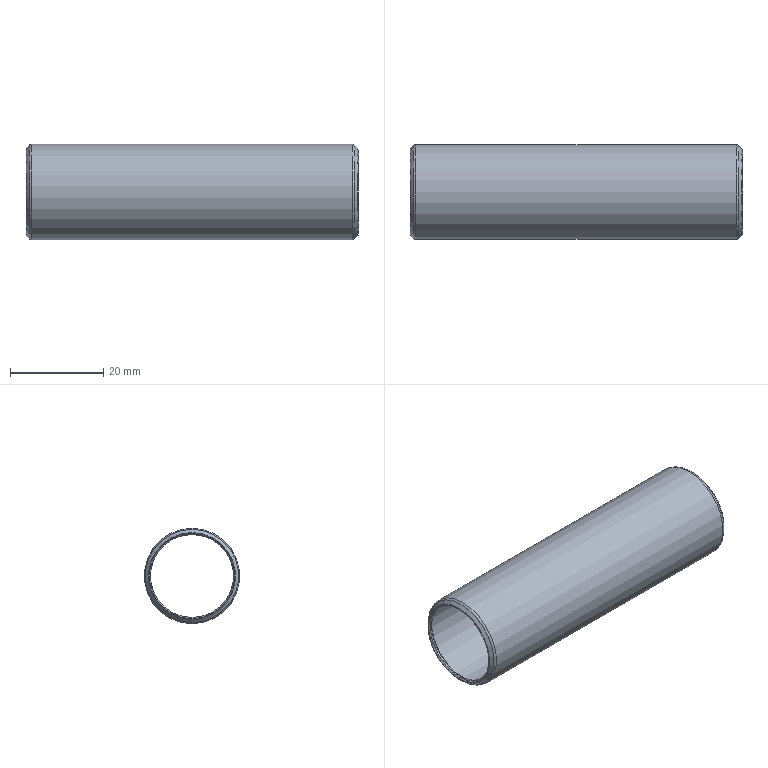Part | NX | features solid 2 | 1 solid | 14 faces | box 71.343 x 20.511 x 20.511 mm | volume 2641 mm3 | cone 6 | cylinder 4 | torus 4 | commonest cylinder face diameters 17.818 x2 19.342 x1 20.511 x1
STEP:
#1=CARTESIAN_POINT('',(69.99,0.,8.909));
#2=VERTEX_POINT('',#1);
#3=CARTESIAN_POINT('',(69.99,0.,0.));
#4=DIRECTION('',(-1.,0.,0.));
#5=DIRECTION('',(0.,0.,1.));
#6=AXIS2_PLACEMENT_3D('',#3,#4,#5);
#7=CIRCLE('',#6,8.909);
#8=EDGE_CURVE('',#2,#2,#7,.T.);
#9=ORIENTED_EDGE('',*,*,#8,.F.);
#10=EDGE_LOOP('',(#9));
#11=FACE_BOUND('',#10,.T.);
#12=CARTESIAN_POINT('',(69.228,0.,9.671));
#13=VERTEX_POINT('',#12);
#14=CARTESIAN_POINT('',(69.228,0.,0.));
#15=DIRECTION('',(-1.,0.,0.));
#16=DIRECTION('',(0.,0.,1.));
#17=AXIS2_PLACEMENT_3D('',#14,#15,#16);
#18=CIRCLE('',#17,9.671);
#19=EDGE_CURVE('',#13,#13,#18,.T.);
#20=ORIENTED_EDGE('',*,*,#19,.T.);
#21=EDGE_LOOP('',(#20));
#22=FACE_BOUND('',#21,.T.);
#23=CARTESIAN_POINT('',(69.228,0.,0.));
#24=DIRECTION('',(-1.,0.,0.));
#25=DIRECTION('',(0.,0.,1.));
#26=AXIS2_PLACEMENT_3D('',#23,#24,#25);
#27=CONICAL_SURFACE('',#26,9.671,0.7854);
#28=ADVANCED_FACE('',(#11,#22),#27,.F.);
#29=CARTESIAN_POINT('',(70.371,0.,8.909));
#30=VERTEX_POINT('',#29);
#31=CARTESIAN_POINT('',(70.371,0.,0.));
#32=DIRECTION('',(-1.,0.,0.));
#33=DIRECTION('',(0.,0.,1.));
#34=AXIS2_PLACEMENT_3D('',#31,#32,#33);
#35=CIRCLE('',#34,8.909);
#36=EDGE_CURVE('',#30,#30,#35,.T.);
#37=ORIENTED_EDGE('',*,*,#36,.F.);
#38=EDGE_LOOP('',(#37));
#39=FACE_BOUND('',#38,.T.);
#40=ORIENTED_EDGE('',*,*,#8,.T.);
#41=EDGE_LOOP('',(#40));
#42=FACE_BOUND('',#41,.T.);
#43=CARTESIAN_POINT('',(69.99,0.,0.));
#44=DIRECTION('',(-1.,0.,0.));
#45=DIRECTION('',(0.,0.,1.));
#46=AXIS2_PLACEMENT_3D('',#43,#44,#45);
#47=CYLINDRICAL_SURFACE('',#46,8.909);
#48=ADVANCED_FACE('',(#39,#42),#47,.F.);
#49=CARTESIAN_POINT('',(70.629,0.,9.168));
#50=VERTEX_POINT('',#49);
#51=CARTESIAN_POINT('',(70.629,0.,0.));
#52=DIRECTION('',(-1.,0.,0.));
#53=DIRECTION('',(0.,0.,1.));
#54=AXIS2_PLACEMENT_3D('',#51,#52,#53);
#55=CIRCLE('',#54,9.168);
#56=EDGE_CURVE('',#50,#50,#55,.T.);
#57=ORIENTED_EDGE('',*,*,#56,.F.);
#58=EDGE_LOOP('',(#57));
#59=FACE_BOUND('',#58,.T.);
#60=ORIENTED_EDGE('',*,*,#36,.T.);
#61=EDGE_LOOP('',(#60));
#62=FACE_BOUND('',#61,.T.);
#63=CARTESIAN_POINT('',(70.371,0.,0.));
#64=DIRECTION('',(1.,0.,0.));
#65=DIRECTION('',(0.,0.,-1.));
#66=AXIS2_PLACEMENT_3D('',#63,#64,#65);
#67=CONICAL_SURFACE('',#66,8.909,0.7854);
#68=ADVANCED_FACE('',(#59,#62),#67,.F.);
#69=ORIENTED_EDGE('',*,*,#56,.T.);
#70=EDGE_LOOP('',(#69));
#71=FACE_BOUND('',#70,.T.);
#72=CARTESIAN_POINT('',(70.629,0.,9.347));
#73=VERTEX_POINT('',#72);
#74=CARTESIAN_POINT('',(70.629,0.,0.));
#75=DIRECTION('',(-1.,0.,0.));
#76=DIRECTION('',(0.,0.,1.));
#77=AXIS2_PLACEMENT_3D('',#74,#75,#76);
#78=CIRCLE('',#77,9.347);
#79=EDGE_CURVE('',#73,#73,#78,.T.);
#80=ORIENTED_EDGE('',*,*,#79,.F.);
#81=EDGE_LOOP('',(#80));
#82=FACE_BOUND('',#81,.T.);
#83=CARTESIAN_POINT('',(70.539,0.,0.));
#84=DIRECTION('',(-1.,0.,0.));
#85=DIRECTION('',(0.,0.,1.));
#86=AXIS2_PLACEMENT_3D('',#83,#84,#85);
#87=TOROIDAL_SURFACE('',#86,9.257,0.127);
#88=ADVANCED_FACE('',(#71,#82),#87,.T.);
#89=CARTESIAN_POINT('',(69.944,0.,10.032));
#90=VERTEX_POINT('',#89);
#91=CARTESIAN_POINT('',(69.944,0.,0.));
#92=DIRECTION('',(-1.,0.,0.));
#93=DIRECTION('',(0.,0.,1.));
#94=AXIS2_PLACEMENT_3D('',#91,#92,#93);
#95=CIRCLE('',#94,10.032);
#96=EDGE_CURVE('',#90,#90,#95,.T.);
#97=ORIENTED_EDGE('',*,*,#96,.F.);
#98=EDGE_LOOP('',(#97));
#99=FACE_BOUND('',#98,.T.);
#100=ORIENTED_EDGE('',*,*,#79,.T.);
#101=EDGE_LOOP('',(#100));
#102=FACE_BOUND('',#101,.T.);
#103=CARTESIAN_POINT('',(70.629,0.,0.));
#104=DIRECTION('',(-1.,0.,0.));
#105=DIRECTION('',(0.,0.,1.));
#106=AXIS2_PLACEMENT_3D('',#103,#104,#105);
#107=CONICAL_SURFACE('',#106,9.347,0.7854);
#108=ADVANCED_FACE('',(#99,#102),#107,.T.);
#109=ORIENTED_EDGE('',*,*,#96,.T.);
#110=EDGE_LOOP('',(#109));
#111=FACE_BOUND('',#110,.T.);
#112=CARTESIAN_POINT('',(69.406,0.,10.255));
#113=VERTEX_POINT('',#112);
#114=CARTESIAN_POINT('',(69.406,0.,0.));
#115=DIRECTION('',(-1.,0.,0.));
#116=DIRECTION('',(0.,0.,1.));
#117=AXIS2_PLACEMENT_3D('',#114,#115,#116);
#118=CIRCLE('',#117,10.255);
#119=EDGE_CURVE('',#113,#113,#118,.T.);
#120=ORIENTED_EDGE('',*,*,#119,.F.);
#121=EDGE_LOOP('',(#120));
#122=FACE_BOUND('',#121,.T.);
#123=CARTESIAN_POINT('',(69.406,0.,0.));
#124=DIRECTION('',(-1.,0.,0.));
#125=DIRECTION('',(0.,0.,1.));
#126=AXIS2_PLACEMENT_3D('',#123,#124,#125);
#127=TOROIDAL_SURFACE('',#126,9.493,0.762);
#128=ADVANCED_FACE('',(#111,#122),#127,.T.);
#129=CARTESIAN_POINT('',(0.5842,0.,10.255));
#130=VERTEX_POINT('',#129);
#131=CARTESIAN_POINT('',(0.5842,0.,0.));
#132=DIRECTION('',(-1.,0.,0.));
#133=DIRECTION('',(0.,0.,1.));
#134=AXIS2_PLACEMENT_3D('',#131,#132,#133);
#135=CIRCLE('',#134,10.255);
#136=EDGE_CURVE('',#130,#130,#135,.T.);
#137=ORIENTED_EDGE('',*,*,#136,.F.);
#138=EDGE_LOOP('',(#137));
#139=FACE_BOUND('',#138,.T.);
#140=ORIENTED_EDGE('',*,*,#119,.T.);
#141=EDGE_LOOP('',(#140));
#142=FACE_BOUND('',#141,.T.);
#143=CARTESIAN_POINT('',(69.99,0.,0.));
#144=DIRECTION('',(-1.,0.,0.));
#145=DIRECTION('',(0.,0.,1.));
#146=AXIS2_PLACEMENT_3D('',#143,#144,#145);
#147=CYLINDRICAL_SURFACE('',#146,10.255);
#148=ADVANCED_FACE('',(#139,#142),#147,.T.);
#149=ORIENTED_EDGE('',*,*,#136,.T.);
#150=EDGE_LOOP('',(#149));
#151=FACE_BOUND('',#150,.T.);
#152=CARTESIAN_POINT('',(0.04538,0.,10.032));
#153=VERTEX_POINT('',#152);
#154=CARTESIAN_POINT('',(0.04538,0.,0.));
#155=DIRECTION('',(-1.,0.,0.));
#156=DIRECTION('',(0.,0.,1.));
#157=AXIS2_PLACEMENT_3D('',#154,#155,#156);
#158=CIRCLE('',#157,10.032);
#159=EDGE_CURVE('',#153,#153,#158,.T.);
#160=ORIENTED_EDGE('',*,*,#159,.F.);
#161=EDGE_LOOP('',(#160));
#162=FACE_BOUND('',#161,.T.);
#163=CARTESIAN_POINT('',(0.5842,0.,0.));
#164=DIRECTION('',(-1.,0.,0.));
#165=DIRECTION('',(0.,0.,1.));
#166=AXIS2_PLACEMENT_3D('',#163,#164,#165);
#167=TOROIDAL_SURFACE('',#166,9.493,0.762);
#168=ADVANCED_FACE('',(#151,#162),#167,.T.);
#169=CARTESIAN_POINT('',(-0.6395,0.,9.347));
#170=VERTEX_POINT('',#169);
#171=CARTESIAN_POINT('',(-0.6395,0.,0.));
#172=DIRECTION('',(-1.,0.,0.));
#173=DIRECTION('',(0.,0.,1.));
#174=AXIS2_PLACEMENT_3D('',#171,#172,#173);
#175=CIRCLE('',#174,9.347);
#176=EDGE_CURVE('',#170,#170,#175,.T.);
#177=ORIENTED_EDGE('',*,*,#176,.F.);
#178=EDGE_LOOP('',(#177));
#179=FACE_BOUND('',#178,.T.);
#180=ORIENTED_EDGE('',*,*,#159,.T.);
#181=EDGE_LOOP('',(#180));
#182=FACE_BOUND('',#181,.T.);
#183=CARTESIAN_POINT('',(0.04538,0.,0.));
#184=DIRECTION('',(1.,0.,0.));
#185=DIRECTION('',(0.,0.,-1.));
#186=AXIS2_PLACEMENT_3D('',#183,#184,#185);
#187=CONICAL_SURFACE('',#186,10.032,0.7854);
#188=ADVANCED_FACE('',(#179,#182),#187,.T.);
#189=ORIENTED_EDGE('',*,*,#176,.T.);
#190=EDGE_LOOP('',(#189));
#191=FACE_BOUND('',#190,.T.);
#192=CARTESIAN_POINT('',(-0.6395,0.,9.168));
#193=VERTEX_POINT('',#192);
#194=CARTESIAN_POINT('',(-0.6395,0.,0.));
#195=DIRECTION('',(-1.,0.,0.));
#196=DIRECTION('',(0.,0.,1.));
#197=AXIS2_PLACEMENT_3D('',#194,#195,#196);
#198=CIRCLE('',#197,9.168);
#199=EDGE_CURVE('',#193,#193,#198,.T.);
#200=ORIENTED_EDGE('',*,*,#199,.F.);
#201=EDGE_LOOP('',(#200));
#202=FACE_BOUND('',#201,.T.);
#203=CARTESIAN_POINT('',(-0.5497,0.,0.));
#204=DIRECTION('',(-1.,0.,0.));
#205=DIRECTION('',(0.,0.,1.));
#206=AXIS2_PLACEMENT_3D('',#203,#204,#205);
#207=TOROIDAL_SURFACE('',#206,9.257,0.127);
#208=ADVANCED_FACE('',(#191,#202),#207,.T.);
#209=CARTESIAN_POINT('',(-0.381,0.,8.909));
#210=VERTEX_POINT('',#209);
#211=CARTESIAN_POINT('',(-0.381,0.,0.));
#212=DIRECTION('',(-1.,0.,0.));
#213=DIRECTION('',(0.,0.,1.));
#214=AXIS2_PLACEMENT_3D('',#211,#212,#213);
#215=CIRCLE('',#214,8.909);
#216=EDGE_CURVE('',#210,#210,#215,.T.);
#217=ORIENTED_EDGE('',*,*,#216,.F.);
#218=EDGE_LOOP('',(#217));
#219=FACE_BOUND('',#218,.T.);
#220=ORIENTED_EDGE('',*,*,#199,.T.);
#221=EDGE_LOOP('',(#220));
#222=FACE_BOUND('',#221,.T.);
#223=CARTESIAN_POINT('',(-0.6395,0.,0.));
#224=DIRECTION('',(-1.,0.,0.));
#225=DIRECTION('',(0.,0.,1.));
#226=AXIS2_PLACEMENT_3D('',#223,#224,#225);
#227=CONICAL_SURFACE('',#226,9.168,0.7854);
#228=ADVANCED_FACE('',(#219,#222),#227,.F.);
#229=CARTESIAN_POINT('',(0.,0.,8.909));
#230=VERTEX_POINT('',#229);
#231=CARTESIAN_POINT('',(0.,0.,0.));
#232=DIRECTION('',(-1.,0.,0.));
#233=DIRECTION('',(0.,0.,1.));
#234=AXIS2_PLACEMENT_3D('',#231,#232,#233);
#235=CIRCLE('',#234,8.909);
#236=EDGE_CURVE('',#230,#230,#235,.T.);
#237=ORIENTED_EDGE('',*,*,#236,.F.);
#238=EDGE_LOOP('',(#237));
#239=FACE_BOUND('',#238,.T.);
#240=ORIENTED_EDGE('',*,*,#216,.T.);
#241=EDGE_LOOP('',(#240));
#242=FACE_BOUND('',#241,.T.);
#243=CARTESIAN_POINT('',(69.99,0.,0.));
#244=DIRECTION('',(-1.,0.,0.));
#245=DIRECTION('',(0.,0.,1.));
#246=AXIS2_PLACEMENT_3D('',#243,#244,#245);
#247=CYLINDRICAL_SURFACE('',#246,8.909);
#248=ADVANCED_FACE('',(#239,#242),#247,.F.);
#249=CARTESIAN_POINT('',(0.762,0.,9.671));
#250=VERTEX_POINT('',#249);
#251=CARTESIAN_POINT('',(0.762,0.,0.));
#252=DIRECTION('',(-1.,0.,0.));
#253=DIRECTION('',(0.,0.,1.));
#254=AXIS2_PLACEMENT_3D('',#251,#252,#253);
#255=CIRCLE('',#254,9.671);
#256=EDGE_CURVE('',#250,#250,#255,.T.);
#257=ORIENTED_EDGE('',*,*,#256,.F.);
#258=EDGE_LOOP('',(#257));
#259=FACE_BOUND('',#258,.T.);
#260=ORIENTED_EDGE('',*,*,#236,.T.);
#261=EDGE_LOOP('',(#260));
#262=FACE_BOUND('',#261,.T.);
#263=CARTESIAN_POINT('',(0.,0.,0.));
#264=DIRECTION('',(1.,0.,0.));
#265=DIRECTION('',(0.,0.,-1.));
#266=AXIS2_PLACEMENT_3D('',#263,#264,#265);
#267=CONICAL_SURFACE('',#266,8.909,0.7854);
#268=ADVANCED_FACE('',(#259,#262),#267,.F.);
#269=ORIENTED_EDGE('',*,*,#19,.F.);
#270=EDGE_LOOP('',(#269));
#271=FACE_BOUND('',#270,.T.);
#272=ORIENTED_EDGE('',*,*,#256,.T.);
#273=EDGE_LOOP('',(#272));
#274=FACE_BOUND('',#273,.T.);
#275=CARTESIAN_POINT('',(69.99,0.,0.));
#276=DIRECTION('',(-1.,0.,0.));
#277=DIRECTION('',(0.,0.,1.));
#278=AXIS2_PLACEMENT_3D('',#275,#276,#277);
#279=CYLINDRICAL_SURFACE('',#278,9.671);
#280=ADVANCED_FACE('',(#271,#274),#279,.F.);
#281=CLOSED_SHELL('',(#28,#48,#68,#88,#108,#128,#148,#168,#188,#208,#228,#248,#268,#280));
#282=MANIFOLD_SOLID_BREP('',#281);
#283=(LENGTH_UNIT()NAMED_UNIT(*)SI_UNIT(.MILLI.,.METRE.));
#284=UNCERTAINTY_MEASURE_WITH_UNIT(LENGTH_MEASURE(0.00001),#283,'','');
#285=(NAMED_UNIT(*)PLANE_ANGLE_UNIT()SI_UNIT($,.RADIAN.));
#286=(NAMED_UNIT(*)SI_UNIT($,.STERADIAN.)SOLID_ANGLE_UNIT());
#287=(GEOMETRIC_REPRESENTATION_CONTEXT(3)GLOBAL_UNCERTAINTY_ASSIGNED_CONTEXT((#284))GLOBAL_UNIT_ASSIGNED_CONTEXT((#283,#285,#286))REPRESENTATION_CONTEXT('',''));
#288=ADVANCED_BREP_SHAPE_REPRESENTATION('',(#282),#287);